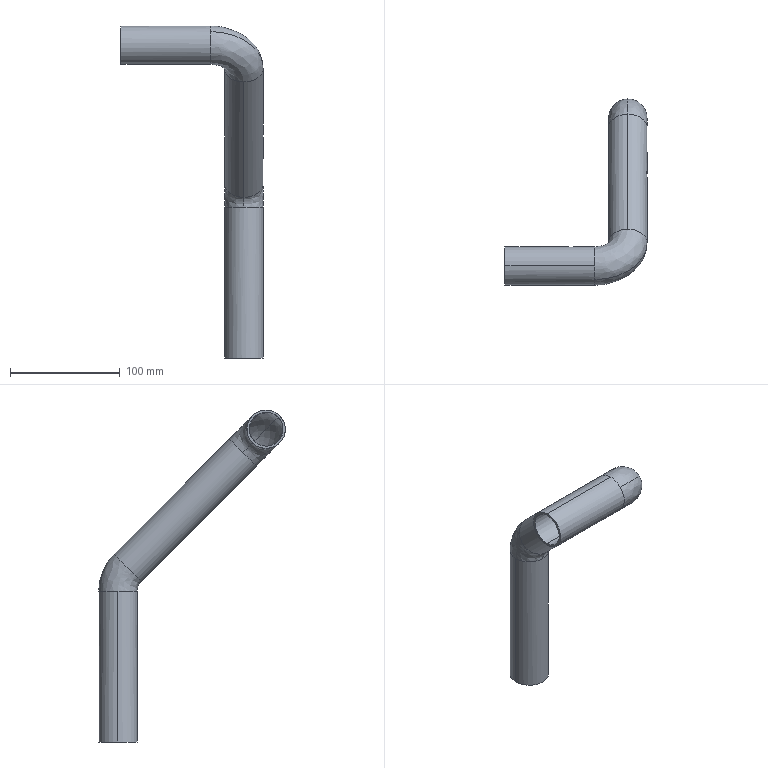Part | STEP file | copper tube 2_default_machined_ | 1 solid | 26 faces | box 129.5 x 170 x 302.5 mm | volume 90840 mm3 | cylinder 16 | spline 8 | plane 2 | commonest cylinder face diameters 31 x6 35 x6 6.5 x4